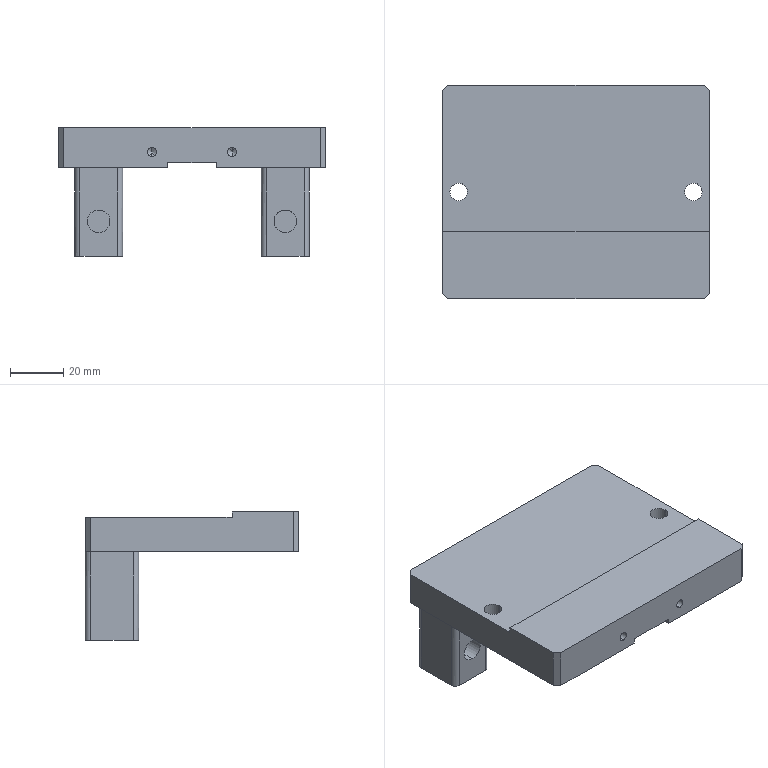NC program | NX | posted with a generic post | part box 100 x 80 x 48 mm
Whole program, first 1415 of 1793 lines:
N10 G17 G21 G94 G90
(FLOOR_WALL , TOOL : D80)
N12 T19 M6
N14 G54
N16 G17 G0 G90 X-95. Y41.997 S6500 M3
N18 G43 Z30. H19
N20 Z3.
N22 G94 G1 Z0. F1500.
N24 X-92.
N26 X92.
N28 Y15.999
N30 X-92.
N32 Y-10.
N34 X92.
N36 X95.
N38 Z3.
N40 G0 Z30.
N42 M5
(ZLEVEL_PROFILE , TOOL : D10)
N44 T15 M6
N46 G54
N48 G17 G0 G90 X47.703 Y-45.1 S9500 M3
N50 G43 Z30. H15
N52 Z1.5
N54 G94 G1 X0. Z-1. F1000.
N56 X-48. F3000.
N58 G2 X-51.606 Y-43.606 R5.1
N60 G1 X-53.606 Y-41.606
N62 G2 X-55.1 Y-38. R5.1
N64 G1 Y38.
N66 G2 X-53.606 Y41.606 R5.1
N68 G1 X-51.606 Y43.606
N70 G2 X-48. Y45.1 R5.1
N72 G1 X48.
N74 G2 X51.606 Y43.606 R5.1
N76 G1 X53.606 Y41.606
N78 G2 X55.1 Y38. R5.1
N80 G1 Y-38.
N82 G2 X53.606 Y-41.606 R5.1
N84 G1 X51.606 Y-43.606
N86 G2 X48. Y-45.1 R5.1
N88 G1 X0.
N90 X-48. Z-1.124
N92 X-48.5 Y-45.075 Z-1.125
N94 X-48.995 Y-45.002 Z-1.127
N96 X-49.48 Y-44.88 Z-1.128
N98 X-49.952 Y-44.712 Z-1.129
N100 X-50.404 Y-44.498 Z-1.13
N102 X-50.833 Y-44.24 Z-1.132
N104 X-51.235 Y-43.942 Z-1.133
N106 X-51.606 Y-43.606 Z-1.134
N108 X-53.606 Y-41.606 Z-1.142
N110 X-53.942 Y-41.235 Z-1.143
N112 X-54.24 Y-40.833 Z-1.144
N114 X-54.498 Y-40.404 Z-1.145
N116 X-54.712 Y-39.952 Z-1.147
N118 X-54.88 Y-39.48 Z-1.148
N120 X-55.002 Y-38.995 Z-1.149
N122 X-55.075 Y-38.5 Z-1.151
N124 X-55.1 Y-38. Z-1.152
N126 Y38. Z-1.348
N128 X-55.075 Y38.5 Z-1.349
N130 X-55.002 Y38.995 Z-1.351
N132 X-54.88 Y39.48 Z-1.352
N134 X-54.712 Y39.952 Z-1.353
N136 X-54.498 Y40.404 Z-1.355
N138 X-54.24 Y40.833 Z-1.356
N140 X-53.942 Y41.235 Z-1.357
N142 X-53.606 Y41.606 Z-1.358
N144 X-51.606 Y43.606 Z-1.366
N146 X-51.235 Y43.942 Z-1.367
N148 X-50.833 Y44.24 Z-1.368
N150 X-50.404 Y44.498 Z-1.37
N152 X-49.952 Y44.712 Z-1.371
N154 X-49.48 Y44.88 Z-1.372
N156 X-48.995 Y45.002 Z-1.373
N158 X-48.5 Y45.075 Z-1.375
N160 X-48. Y45.1 Z-1.376
N162 X48. Z-1.624
N164 X48.5 Y45.075 Z-1.625
N166 X48.995 Y45.002 Z-1.627
N168 X49.48 Y44.88 Z-1.628
N170 X49.952 Y44.712 Z-1.629
N172 X50.404 Y44.498 Z-1.63
N174 X50.833 Y44.24 Z-1.632
N176 X51.235 Y43.942 Z-1.633
N178 X51.606 Y43.606 Z-1.634
N180 X53.606 Y41.606 Z-1.642
N182 X53.942 Y41.235 Z-1.643
N184 X54.24 Y40.833 Z-1.644
N186 X54.498 Y40.404 Z-1.645
N188 X54.712 Y39.952 Z-1.647
N190 X54.88 Y39.48 Z-1.648
N192 X55.002 Y38.995 Z-1.649
N194 X55.075 Y38.5 Z-1.651
N196 X55.1 Y38. Z-1.652
N198 Y-38. Z-1.848
N200 X55.075 Y-38.5 Z-1.849
N202 X55.002 Y-38.995 Z-1.851
N204 X54.88 Y-39.48 Z-1.852
N206 X54.712 Y-39.952 Z-1.853
N208 X54.498 Y-40.404 Z-1.855
N210 X54.24 Y-40.833 Z-1.856
N212 X53.942 Y-41.235 Z-1.857
N214 X53.606 Y-41.606 Z-1.858
N216 X51.606 Y-43.606 Z-1.866
N218 X51.235 Y-43.942 Z-1.867
N220 X50.833 Y-44.24 Z-1.868
N222 X50.404 Y-44.498 Z-1.87
N224 X49.952 Y-44.712 Z-1.871
N226 X49.48 Y-44.88 Z-1.872
N228 X48.995 Y-45.002 Z-1.873
N230 X48.5 Y-45.075 Z-1.875
N232 X48. Y-45.1 Z-1.876
N234 X0. Z-2.
N236 X-48. Z-2.124
N238 X-48.5 Y-45.075 Z-2.125
N240 X-48.995 Y-45.002 Z-2.127
N242 X-49.48 Y-44.88 Z-2.128
N244 X-49.952 Y-44.712 Z-2.129
N246 X-50.404 Y-44.498 Z-2.13
N248 X-50.833 Y-44.24 Z-2.132
N250 X-51.235 Y-43.942 Z-2.133
N252 X-51.606 Y-43.606 Z-2.134
N254 X-53.606 Y-41.606 Z-2.142
N256 X-53.942 Y-41.235 Z-2.143
N258 X-54.24 Y-40.833 Z-2.144
N260 X-54.498 Y-40.404 Z-2.145
N262 X-54.712 Y-39.952 Z-2.147
N264 X-54.88 Y-39.48 Z-2.148
N266 X-55.002 Y-38.995 Z-2.149
N268 X-55.075 Y-38.5 Z-2.151
N270 X-55.1 Y-38. Z-2.152
N272 Y38. Z-2.348
N274 X-55.075 Y38.5 Z-2.349
N276 X-55.002 Y38.995 Z-2.351
N278 X-54.88 Y39.48 Z-2.352
N280 X-54.712 Y39.952 Z-2.353
N282 X-54.498 Y40.404 Z-2.355
N284 X-54.24 Y40.833 Z-2.356
N286 X-53.942 Y41.235 Z-2.357
N288 X-53.606 Y41.606 Z-2.358
N290 X-51.606 Y43.606 Z-2.366
N292 X-51.235 Y43.942 Z-2.367
N294 X-50.833 Y44.24 Z-2.368
N296 X-50.404 Y44.498 Z-2.37
N298 X-49.952 Y44.712 Z-2.371
N300 X-49.48 Y44.88 Z-2.372
N302 X-48.995 Y45.002 Z-2.373
N304 X-48.5 Y45.075 Z-2.375
N306 X-48. Y45.1 Z-2.376
N308 X48. Z-2.624
N310 X48.5 Y45.075 Z-2.625
N312 X48.995 Y45.002 Z-2.627
N314 X49.48 Y44.88 Z-2.628
N316 X49.952 Y44.712 Z-2.629
N318 X50.404 Y44.498 Z-2.63
N320 X50.833 Y44.24 Z-2.632
N322 X51.235 Y43.942 Z-2.633
N324 X51.606 Y43.606 Z-2.634
N326 X53.606 Y41.606 Z-2.642
N328 X53.942 Y41.235 Z-2.643
N330 X54.24 Y40.833 Z-2.644
N332 X54.498 Y40.404 Z-2.645
N334 X54.712 Y39.952 Z-2.647
N336 X54.88 Y39.48 Z-2.648
N338 X55.002 Y38.995 Z-2.649
N340 X55.075 Y38.5 Z-2.651
N342 X55.1 Y38. Z-2.652
N344 Y-38. Z-2.848
N346 X55.075 Y-38.5 Z-2.849
N348 X55.002 Y-38.995 Z-2.851
N350 X54.88 Y-39.48 Z-2.852
N352 X54.712 Y-39.952 Z-2.853
N354 X54.498 Y-40.404 Z-2.855
N356 X54.24 Y-40.833 Z-2.856
N358 X53.942 Y-41.235 Z-2.857
N360 X53.606 Y-41.606 Z-2.858
N362 X51.606 Y-43.606 Z-2.866
N364 X51.235 Y-43.942 Z-2.867
N366 X50.833 Y-44.24 Z-2.868
N368 X50.404 Y-44.498 Z-2.87
N370 X49.952 Y-44.712 Z-2.871
N372 X49.48 Y-44.88 Z-2.872
N374 X48.995 Y-45.002 Z-2.873
N376 X48.5 Y-45.075 Z-2.875
N378 X48. Y-45.1 Z-2.876
N380 X0. Z-3.
N382 X-48. Z-3.124
N384 X-48.5 Y-45.075 Z-3.125
N386 X-48.995 Y-45.002 Z-3.127
N388 X-49.48 Y-44.88 Z-3.128
N390 X-49.952 Y-44.712 Z-3.129
N392 X-50.404 Y-44.498 Z-3.13
N394 X-50.833 Y-44.24 Z-3.132
N396 X-51.235 Y-43.942 Z-3.133
N398 X-51.606 Y-43.606 Z-3.134
N400 X-53.606 Y-41.606 Z-3.142
N402 X-53.942 Y-41.235 Z-3.143
N404 X-54.24 Y-40.833 Z-3.144
N406 X-54.498 Y-40.404 Z-3.145
N408 X-54.712 Y-39.952 Z-3.147
N410 X-54.88 Y-39.48 Z-3.148
N412 X-55.002 Y-38.995 Z-3.149
N414 X-55.075 Y-38.5 Z-3.151
N416 X-55.1 Y-38. Z-3.152
N418 Y38. Z-3.348
N420 X-55.075 Y38.5 Z-3.349
N422 X-55.002 Y38.995 Z-3.351
N424 X-54.88 Y39.48 Z-3.352
N426 X-54.712 Y39.952 Z-3.353
N428 X-54.498 Y40.404 Z-3.355
N430 X-54.24 Y40.833 Z-3.356
N432 X-53.942 Y41.235 Z-3.357
N434 X-53.606 Y41.606 Z-3.358
N436 X-51.606 Y43.606 Z-3.366
N438 X-51.235 Y43.942 Z-3.367
N440 X-50.833 Y44.24 Z-3.368
N442 X-50.404 Y44.498 Z-3.37
N444 X-49.952 Y44.712 Z-3.371
N446 X-49.48 Y44.88 Z-3.372
N448 X-48.995 Y45.002 Z-3.373
N450 X-48.5 Y45.075 Z-3.375
N452 X-48. Y45.1 Z-3.376
N454 X48. Z-3.624
N456 X48.5 Y45.075 Z-3.625
N458 X48.995 Y45.002 Z-3.627
N460 X49.48 Y44.88 Z-3.628
N462 X49.952 Y44.712 Z-3.629
N464 X50.404 Y44.498 Z-3.63
N466 X50.833 Y44.24 Z-3.632
N468 X51.235 Y43.942 Z-3.633
N470 X51.606 Y43.606 Z-3.634
N472 X53.606 Y41.606 Z-3.642
N474 X53.942 Y41.235 Z-3.643
N476 X54.24 Y40.833 Z-3.644
N478 X54.498 Y40.404 Z-3.645
N480 X54.712 Y39.952 Z-3.647
N482 X54.88 Y39.48 Z-3.648
N484 X55.002 Y38.995 Z-3.649
N486 X55.075 Y38.5 Z-3.651
N488 X55.1 Y38. Z-3.652
N490 Y-38. Z-3.848
N492 X55.075 Y-38.5 Z-3.849
N494 X55.002 Y-38.995 Z-3.851
N496 X54.88 Y-39.48 Z-3.852
N498 X54.712 Y-39.952 Z-3.853
N500 X54.498 Y-40.404 Z-3.855
N502 X54.24 Y-40.833 Z-3.856
N504 X53.942 Y-41.235 Z-3.857
N506 X53.606 Y-41.606 Z-3.858
N508 X51.606 Y-43.606 Z-3.866
N510 X51.235 Y-43.942 Z-3.867
N512 X50.833 Y-44.24 Z-3.868
N514 X50.404 Y-44.498 Z-3.87
N516 X49.952 Y-44.712 Z-3.871
N518 X49.48 Y-44.88 Z-3.872
N520 X48.995 Y-45.002 Z-3.873
N522 X48.5 Y-45.075 Z-3.875
N524 X48. Y-45.1 Z-3.876
N526 X0. Z-4.
N528 X-48. Z-4.124
N530 X-48.5 Y-45.075 Z-4.125
N532 X-48.995 Y-45.002 Z-4.127
N534 X-49.48 Y-44.88 Z-4.128
N536 X-49.952 Y-44.712 Z-4.129
N538 X-50.404 Y-44.498 Z-4.13
N540 X-50.833 Y-44.24 Z-4.132
N542 X-51.235 Y-43.942 Z-4.133
N544 X-51.606 Y-43.606 Z-4.134
N546 X-53.606 Y-41.606 Z-4.142
N548 X-53.942 Y-41.235 Z-4.143
N550 X-54.24 Y-40.833 Z-4.144
N552 X-54.498 Y-40.404 Z-4.145
N554 X-54.712 Y-39.952 Z-4.147
N556 X-54.88 Y-39.48 Z-4.148
N558 X-55.002 Y-38.995 Z-4.149
N560 X-55.075 Y-38.5 Z-4.151
N562 X-55.1 Y-38. Z-4.152
N564 Y38. Z-4.348
N566 X-55.075 Y38.5 Z-4.349
N568 X-55.002 Y38.995 Z-4.351
N570 X-54.88 Y39.48 Z-4.352
N572 X-54.712 Y39.952 Z-4.353
N574 X-54.498 Y40.404 Z-4.355
N576 X-54.24 Y40.833 Z-4.356
N578 X-53.942 Y41.235 Z-4.357
N580 X-53.606 Y41.606 Z-4.358
N582 X-51.606 Y43.606 Z-4.366
N584 X-51.235 Y43.942 Z-4.367
N586 X-50.833 Y44.24 Z-4.368
N588 X-50.404 Y44.498 Z-4.37
N590 X-49.952 Y44.712 Z-4.371
N592 X-49.48 Y44.88 Z-4.372
N594 X-48.995 Y45.002 Z-4.373
N596 X-48.5 Y45.075 Z-4.375
N598 X-48. Y45.1 Z-4.376
N600 X48. Z-4.624
N602 X48.5 Y45.075 Z-4.625
N604 X48.995 Y45.002 Z-4.627
N606 X49.48 Y44.88 Z-4.628
N608 X49.952 Y44.712 Z-4.629
N610 X50.404 Y44.498 Z-4.63
N612 X50.833 Y44.24 Z-4.632
N614 X51.235 Y43.942 Z-4.633
N616 X51.606 Y43.606 Z-4.634
N618 X53.606 Y41.606 Z-4.642
N620 X53.942 Y41.235 Z-4.643
N622 X54.24 Y40.833 Z-4.644
N624 X54.498 Y40.404 Z-4.645
N626 X54.712 Y39.952 Z-4.647
N628 X54.88 Y39.48 Z-4.648
N630 X55.002 Y38.995 Z-4.649
N632 X55.075 Y38.5 Z-4.651
N634 X55.1 Y38. Z-4.652
N636 Y-38. Z-4.848
N638 X55.075 Y-38.5 Z-4.849
N640 X55.002 Y-38.995 Z-4.851
N642 X54.88 Y-39.48 Z-4.852
N644 X54.712 Y-39.952 Z-4.853
N646 X54.498 Y-40.404 Z-4.855
N648 X54.24 Y-40.833 Z-4.856
N650 X53.942 Y-41.235 Z-4.857
N652 X53.606 Y-41.606 Z-4.858
N654 X51.606 Y-43.606 Z-4.866
N656 X51.235 Y-43.942 Z-4.867
N658 X50.833 Y-44.24 Z-4.868
N660 X50.404 Y-44.498 Z-4.87
N662 X49.952 Y-44.712 Z-4.871
N664 X49.48 Y-44.88 Z-4.872
N666 X48.995 Y-45.002 Z-4.873
N668 X48.5 Y-45.075 Z-4.875
N670 X48. Y-45.1 Z-4.876
N672 X0. Z-5.
N674 X-48. Z-5.124
N676 X-48.5 Y-45.075 Z-5.125
N678 X-48.995 Y-45.002 Z-5.127
N680 X-49.48 Y-44.88 Z-5.128
N682 X-49.952 Y-44.712 Z-5.129
N684 X-50.404 Y-44.498 Z-5.13
N686 X-50.833 Y-44.24 Z-5.132
N688 X-51.235 Y-43.942 Z-5.133
N690 X-51.606 Y-43.606 Z-5.134
N692 X-53.606 Y-41.606 Z-5.142
N694 X-53.942 Y-41.235 Z-5.143
N696 X-54.24 Y-40.833 Z-5.144
N698 X-54.498 Y-40.404 Z-5.145
N700 X-54.712 Y-39.952 Z-5.147
N702 X-54.88 Y-39.48 Z-5.148
N704 X-55.002 Y-38.995 Z-5.149
N706 X-55.075 Y-38.5 Z-5.151
N708 X-55.1 Y-38. Z-5.152
N710 Y38. Z-5.348
N712 X-55.075 Y38.5 Z-5.349
N714 X-55.002 Y38.995 Z-5.351
N716 X-54.88 Y39.48 Z-5.352
N718 X-54.712 Y39.952 Z-5.353
N720 X-54.498 Y40.404 Z-5.355
N722 X-54.24 Y40.833 Z-5.356
N724 X-53.942 Y41.235 Z-5.357
N726 X-53.606 Y41.606 Z-5.358
N728 X-51.606 Y43.606 Z-5.366
N730 X-51.235 Y43.942 Z-5.367
N732 X-50.833 Y44.24 Z-5.368
N734 X-50.404 Y44.498 Z-5.37
N736 X-49.952 Y44.712 Z-5.371
N738 X-49.48 Y44.88 Z-5.372
N740 X-48.995 Y45.002 Z-5.373
N742 X-48.5 Y45.075 Z-5.375
N744 X-48. Y45.1 Z-5.376
N746 X48. Z-5.624
N748 X48.5 Y45.075 Z-5.625
N750 X48.995 Y45.002 Z-5.627
N752 X49.48 Y44.88 Z-5.628
N754 X49.952 Y44.712 Z-5.629
N756 X50.404 Y44.498 Z-5.63
N758 X50.833 Y44.24 Z-5.632
N760 X51.235 Y43.942 Z-5.633
N762 X51.606 Y43.606 Z-5.634
N764 X53.606 Y41.606 Z-5.642
N766 X53.942 Y41.235 Z-5.643
N768 X54.24 Y40.833 Z-5.644
N770 X54.498 Y40.404 Z-5.645
N772 X54.712 Y39.952 Z-5.647
N774 X54.88 Y39.48 Z-5.648
N776 X55.002 Y38.995 Z-5.649
N778 X55.075 Y38.5 Z-5.651
N780 X55.1 Y38. Z-5.652
N782 Y-38. Z-5.848
N784 X55.075 Y-38.5 Z-5.849
N786 X55.002 Y-38.995 Z-5.851
N788 X54.88 Y-39.48 Z-5.852
N790 X54.712 Y-39.952 Z-5.853
N792 X54.498 Y-40.404 Z-5.855
N794 X54.24 Y-40.833 Z-5.856
N796 X53.942 Y-41.235 Z-5.857
N798 X53.606 Y-41.606 Z-5.858
N800 X51.606 Y-43.606 Z-5.866
N802 X51.235 Y-43.942 Z-5.867
N804 X50.833 Y-44.24 Z-5.868
N806 X50.404 Y-44.498 Z-5.87
N808 X49.952 Y-44.712 Z-5.871
N810 X49.48 Y-44.88 Z-5.872
N812 X48.995 Y-45.002 Z-5.873
N814 X48.5 Y-45.075 Z-5.875
N816 X48. Y-45.1 Z-5.876
N818 X0. Z-6.
N820 X-48. Z-6.124
N822 X-48.5 Y-45.075 Z-6.125
N824 X-48.995 Y-45.002 Z-6.127
N826 X-49.48 Y-44.88 Z-6.128
N828 X-49.952 Y-44.712 Z-6.129
N830 X-50.404 Y-44.498 Z-6.13
N832 X-50.833 Y-44.24 Z-6.132
N834 X-51.235 Y-43.942 Z-6.133
N836 X-51.606 Y-43.606 Z-6.134
N838 X-53.606 Y-41.606 Z-6.142
N840 X-53.942 Y-41.235 Z-6.143
N842 X-54.24 Y-40.833 Z-6.144
N844 X-54.498 Y-40.404 Z-6.145
N846 X-54.712 Y-39.952 Z-6.147
N848 X-54.88 Y-39.48 Z-6.148
N850 X-55.002 Y-38.995 Z-6.149
N852 X-55.075 Y-38.5 Z-6.151
N854 X-55.1 Y-38. Z-6.152
N856 Y38. Z-6.348
N858 X-55.075 Y38.5 Z-6.349
N860 X-55.002 Y38.995 Z-6.351
N862 X-54.88 Y39.48 Z-6.352
N864 X-54.712 Y39.952 Z-6.353
N866 X-54.498 Y40.404 Z-6.355
N868 X-54.24 Y40.833 Z-6.356
N870 X-53.942 Y41.235 Z-6.357
N872 X-53.606 Y41.606 Z-6.358
N874 X-51.606 Y43.606 Z-6.366
N876 X-51.235 Y43.942 Z-6.367
N878 X-50.833 Y44.24 Z-6.368
N880 X-50.404 Y44.498 Z-6.37
N882 X-49.952 Y44.712 Z-6.371
N884 X-49.48 Y44.88 Z-6.372
N886 X-48.995 Y45.002 Z-6.373
N888 X-48.5 Y45.075 Z-6.375
N890 X-48. Y45.1 Z-6.376
N892 X48. Z-6.624
N894 X48.5 Y45.075 Z-6.625
N896 X48.995 Y45.002 Z-6.627
N898 X49.48 Y44.88 Z-6.628
N900 X49.952 Y44.712 Z-6.629
N902 X50.404 Y44.498 Z-6.63
N904 X50.833 Y44.24 Z-6.632
N906 X51.235 Y43.942 Z-6.633
N908 X51.606 Y43.606 Z-6.634
N910 X53.606 Y41.606 Z-6.642
N912 X53.942 Y41.235 Z-6.643
N914 X54.24 Y40.833 Z-6.644
N916 X54.498 Y40.404 Z-6.645
N918 X54.712 Y39.952 Z-6.647
N920 X54.88 Y39.48 Z-6.648
N922 X55.002 Y38.995 Z-6.649
N924 X55.075 Y38.5 Z-6.651
N926 X55.1 Y38. Z-6.652
N928 Y-38. Z-6.848
N930 X55.075 Y-38.5 Z-6.849
N932 X55.002 Y-38.995 Z-6.851
N934 X54.88 Y-39.48 Z-6.852
N936 X54.712 Y-39.952 Z-6.853
N938 X54.498 Y-40.404 Z-6.855
N940 X54.24 Y-40.833 Z-6.856
N942 X53.942 Y-41.235 Z-6.857
N944 X53.606 Y-41.606 Z-6.858
N946 X51.606 Y-43.606 Z-6.866
N948 X51.235 Y-43.942 Z-6.867
N950 X50.833 Y-44.24 Z-6.868
N952 X50.404 Y-44.498 Z-6.87
N954 X49.952 Y-44.712 Z-6.871
N956 X49.48 Y-44.88 Z-6.872
N958 X48.995 Y-45.002 Z-6.873
N960 X48.5 Y-45.075 Z-6.875
N962 X48. Y-45.1 Z-6.876
N964 X0. Z-7.
N966 X-48. Z-7.124
N968 X-48.5 Y-45.075 Z-7.125
N970 X-48.995 Y-45.002 Z-7.127
N972 X-49.48 Y-44.88 Z-7.128
N974 X-49.952 Y-44.712 Z-7.129
N976 X-50.404 Y-44.498 Z-7.13
N978 X-50.833 Y-44.24 Z-7.132
N980 X-51.235 Y-43.942 Z-7.133
N982 X-51.606 Y-43.606 Z-7.134
N984 X-53.606 Y-41.606 Z-7.142
N986 X-53.942 Y-41.235 Z-7.143
N988 X-54.24 Y-40.833 Z-7.144
N990 X-54.498 Y-40.404 Z-7.145
N992 X-54.712 Y-39.952 Z-7.147
N994 X-54.88 Y-39.48 Z-7.148
N996 X-55.002 Y-38.995 Z-7.149
N998 X-55.075 Y-38.5 Z-7.151
N1000 X-55.1 Y-38. Z-7.152
N1002 Y38. Z-7.348
N1004 X-55.075 Y38.5 Z-7.349
N1006 X-55.002 Y38.995 Z-7.351
N1008 X-54.88 Y39.48 Z-7.352
N1010 X-54.712 Y39.952 Z-7.353
N1012 X-54.498 Y40.404 Z-7.355
N1014 X-54.24 Y40.833 Z-7.356
N1016 X-53.942 Y41.235 Z-7.357
N1018 X-53.606 Y41.606 Z-7.358
N1020 X-51.606 Y43.606 Z-7.366
N1022 X-51.235 Y43.942 Z-7.367
N1024 X-50.833 Y44.24 Z-7.368
N1026 X-50.404 Y44.498 Z-7.37
N1028 X-49.952 Y44.712 Z-7.371
N1030 X-49.48 Y44.88 Z-7.372
N1032 X-48.995 Y45.002 Z-7.373
N1034 X-48.5 Y45.075 Z-7.375
N1036 X-48. Y45.1 Z-7.376
N1038 X48. Z-7.624
N1040 X48.5 Y45.075 Z-7.625
N1042 X48.995 Y45.002 Z-7.627
N1044 X49.48 Y44.88 Z-7.628
N1046 X49.952 Y44.712 Z-7.629
N1048 X50.404 Y44.498 Z-7.63
N1050 X50.833 Y44.24 Z-7.632
N1052 X51.235 Y43.942 Z-7.633
N1054 X51.606 Y43.606 Z-7.634
N1056 X53.606 Y41.606 Z-7.642
N1058 X53.942 Y41.235 Z-7.643
N1060 X54.24 Y40.833 Z-7.644
N1062 X54.498 Y40.404 Z-7.645
N1064 X54.712 Y39.952 Z-7.647
N1066 X54.88 Y39.48 Z-7.648
N1068 X55.002 Y38.995 Z-7.649
N1070 X55.075 Y38.5 Z-7.651
N1072 X55.1 Y38. Z-7.652
N1074 Y-38. Z-7.848
N1076 X55.075 Y-38.5 Z-7.849
N1078 X55.002 Y-38.995 Z-7.851
N1080 X54.88 Y-39.48 Z-7.852
N1082 X54.712 Y-39.952 Z-7.853
N1084 X54.498 Y-40.404 Z-7.855
N1086 X54.24 Y-40.833 Z-7.856
N1088 X53.942 Y-41.235 Z-7.857
N1090 X53.606 Y-41.606 Z-7.858
N1092 X51.606 Y-43.606 Z-7.866
N1094 X51.235 Y-43.942 Z-7.867
N1096 X50.833 Y-44.24 Z-7.868
N1098 X50.404 Y-44.498 Z-7.87
N1100 X49.952 Y-44.712 Z-7.871
N1102 X49.48 Y-44.88 Z-7.872
N1104 X48.995 Y-45.002 Z-7.873
N1106 X48.5 Y-45.075 Z-7.875
N1108 X48. Y-45.1 Z-7.876
N1110 X0. Z-8.
N1112 X-48. Z-8.124
N1114 X-48.5 Y-45.075 Z-8.125
N1116 X-48.995 Y-45.002 Z-8.127
N1118 X-49.48 Y-44.88 Z-8.128
N1120 X-49.952 Y-44.712 Z-8.129
N1122 X-50.404 Y-44.498 Z-8.13
N1124 X-50.833 Y-44.24 Z-8.132
N1126 X-51.235 Y-43.942 Z-8.133
N1128 X-51.606 Y-43.606 Z-8.134
N1130 X-53.606 Y-41.606 Z-8.142
N1132 X-53.942 Y-41.235 Z-8.143
N1134 X-54.24 Y-40.833 Z-8.144
N1136 X-54.498 Y-40.404 Z-8.145
N1138 X-54.712 Y-39.952 Z-8.147
N1140 X-54.88 Y-39.48 Z-8.148
N1142 X-55.002 Y-38.995 Z-8.149
N1144 X-55.075 Y-38.5 Z-8.151
N1146 X-55.1 Y-38. Z-8.152
N1148 Y38. Z-8.348
N1150 X-55.075 Y38.5 Z-8.349
N1152 X-55.002 Y38.995 Z-8.351
N1154 X-54.88 Y39.48 Z-8.352
N1156 X-54.712 Y39.952 Z-8.353
N1158 X-54.498 Y40.404 Z-8.355
N1160 X-54.24 Y40.833 Z-8.356
N1162 X-53.942 Y41.235 Z-8.357
N1164 X-53.606 Y41.606 Z-8.358
N1166 X-51.606 Y43.606 Z-8.366
N1168 X-51.235 Y43.942 Z-8.367
N1170 X-50.833 Y44.24 Z-8.368
N1172 X-50.404 Y44.498 Z-8.37
N1174 X-49.952 Y44.712 Z-8.371
N1176 X-49.48 Y44.88 Z-8.372
N1178 X-48.995 Y45.002 Z-8.373
N1180 X-48.5 Y45.075 Z-8.375
N1182 X-48. Y45.1 Z-8.376
N1184 X48. Z-8.624
N1186 X48.5 Y45.075 Z-8.625
N1188 X48.995 Y45.002 Z-8.627
N1190 X49.48 Y44.88 Z-8.628
N1192 X49.952 Y44.712 Z-8.629
N1194 X50.404 Y44.498 Z-8.63
N1196 X50.833 Y44.24 Z-8.632
N1198 X51.235 Y43.942 Z-8.633
N1200 X51.606 Y43.606 Z-8.634
N1202 X53.606 Y41.606 Z-8.642
N1204 X53.942 Y41.235 Z-8.643
N1206 X54.24 Y40.833 Z-8.644
N1208 X54.498 Y40.404 Z-8.645
N1210 X54.712 Y39.952 Z-8.647
N1212 X54.88 Y39.48 Z-8.648
N1214 X55.002 Y38.995 Z-8.649
N1216 X55.075 Y38.5 Z-8.651
N1218 X55.1 Y38. Z-8.652
N1220 Y-38. Z-8.848
N1222 X55.075 Y-38.5 Z-8.849
N1224 X55.002 Y-38.995 Z-8.851
N1226 X54.88 Y-39.48 Z-8.852
N1228 X54.712 Y-39.952 Z-8.853
N1230 X54.498 Y-40.404 Z-8.855
N1232 X54.24 Y-40.833 Z-8.856
N1234 X53.942 Y-41.235 Z-8.857
N1236 X53.606 Y-41.606 Z-8.858
N1238 X51.606 Y-43.606 Z-8.866
N1240 X51.235 Y-43.942 Z-8.867
N1242 X50.833 Y-44.24 Z-8.868
N1244 X50.404 Y-44.498 Z-8.87
N1246 X49.952 Y-44.712 Z-8.871
N1248 X49.48 Y-44.88 Z-8.872
N1250 X48.995 Y-45.002 Z-8.873
N1252 X48.5 Y-45.075 Z-8.875
N1254 X48. Y-45.1 Z-8.876
N1256 X0. Z-9.
N1258 X-48. Z-9.124
N1260 X-48.5 Y-45.075 Z-9.125
N1262 X-48.995 Y-45.002 Z-9.127
N1264 X-49.48 Y-44.88 Z-9.128
N1266 X-49.952 Y-44.712 Z-9.129
N1268 X-50.404 Y-44.498 Z-9.13
N1270 X-50.833 Y-44.24 Z-9.132
N1272 X-51.235 Y-43.942 Z-9.133
N1274 X-51.606 Y-43.606 Z-9.134
N1276 X-53.606 Y-41.606 Z-9.142
N1278 X-53.942 Y-41.235 Z-9.143
N1280 X-54.24 Y-40.833 Z-9.144
N1282 X-54.498 Y-40.404 Z-9.145
N1284 X-54.712 Y-39.952 Z-9.147
N1286 X-54.88 Y-39.48 Z-9.148
N1288 X-55.002 Y-38.995 Z-9.149
N1290 X-55.075 Y-38.5 Z-9.151
N1292 X-55.1 Y-38. Z-9.152
N1294 Y38. Z-9.348
N1296 X-55.075 Y38.5 Z-9.349
N1298 X-55.002 Y38.995 Z-9.351
N1300 X-54.88 Y39.48 Z-9.352
N1302 X-54.712 Y39.952 Z-9.353
N1304 X-54.498 Y40.404 Z-9.355
N1306 X-54.24 Y40.833 Z-9.356
N1308 X-53.942 Y41.235 Z-9.357
N1310 X-53.606 Y41.606 Z-9.358
N1312 X-51.606 Y43.606 Z-9.366
N1314 X-51.235 Y43.942 Z-9.367
N1316 X-50.833 Y44.24 Z-9.368
N1318 X-50.404 Y44.498 Z-9.37
N1320 X-49.952 Y44.712 Z-9.371
N1322 X-49.48 Y44.88 Z-9.372
N1324 X-48.995 Y45.002 Z-9.373
N1326 X-48.5 Y45.075 Z-9.375
N1328 X-48. Y45.1 Z-9.376
N1330 X48. Z-9.624
N1332 X48.5 Y45.075 Z-9.625
N1334 X48.995 Y45.002 Z-9.627
N1336 X49.48 Y44.88 Z-9.628
N1338 X49.952 Y44.712 Z-9.629
N1340 X50.404 Y44.498 Z-9.63
N1342 X50.833 Y44.24 Z-9.632
N1344 X51.235 Y43.942 Z-9.633
N1346 X51.606 Y43.606 Z-9.634
N1348 X53.606 Y41.606 Z-9.642
N1350 X53.942 Y41.235 Z-9.643
N1352 X54.24 Y40.833 Z-9.644
N1354 X54.498 Y40.404 Z-9.645
N1356 X54.712 Y39.952 Z-9.647
N1358 X54.88 Y39.48 Z-9.648
N1360 X55.002 Y38.995 Z-9.649
N1362 X55.075 Y38.5 Z-9.651
N1364 X55.1 Y38. Z-9.652
N1366 Y-38. Z-9.848
N1368 X55.075 Y-38.5 Z-9.849
N1370 X55.002 Y-38.995 Z-9.851
N1372 X54.88 Y-39.48 Z-9.852
N1374 X54.712 Y-39.952 Z-9.853
N1376 X54.498 Y-40.404 Z-9.855
N1378 X54.24 Y-40.833 Z-9.856
N1380 X53.942 Y-41.235 Z-9.857
N1382 X53.606 Y-41.606 Z-9.858
N1384 X51.606 Y-43.606 Z-9.866
N1386 X51.235 Y-43.942 Z-9.867
N1388 X50.833 Y-44.24 Z-9.868
N1390 X50.404 Y-44.498 Z-9.87
N1392 X49.952 Y-44.712 Z-9.871
N1394 X49.48 Y-44.88 Z-9.872
N1396 X48.995 Y-45.002 Z-9.873
N1398 X48.5 Y-45.075 Z-9.875
N1400 X48. Y-45.1 Z-9.876
N1402 X0. Z-10.
N1404 X-48. Z-10.124
N1406 X-48.5 Y-45.075 Z-10.125
N1408 X-48.995 Y-45.002 Z-10.127
N1410 X-49.48 Y-44.88 Z-10.128
N1412 X-49.952 Y-44.712 Z-10.129
N1414 X-50.404 Y-44.498 Z-10.13
N1416 X-50.833 Y-44.24 Z-10.132
N1418 X-51.235 Y-43.942 Z-10.133
N1420 X-51.606 Y-43.606 Z-10.134
N1422 X-53.606 Y-41.606 Z-10.142
N1424 X-53.942 Y-41.235 Z-10.143
N1426 X-54.24 Y-40.833 Z-10.144
N1428 X-54.498 Y-40.404 Z-10.145
N1430 X-54.712 Y-39.952 Z-10.147
N1432 X-54.88 Y-39.48 Z-10.148
N1434 X-55.002 Y-38.995 Z-10.149
N1436 X-55.075 Y-38.5 Z-10.151
N1438 X-55.1 Y-38. Z-10.152
N1440 Y38. Z-10.348
N1442 X-55.075 Y38.5 Z-10.349
N1444 X-55.002 Y38.995 Z-10.351
N1446 X-54.88 Y39.48 Z-10.352
N1448 X-54.712 Y39.952 Z-10.353
N1450 X-54.498 Y40.404 Z-10.355
N1452 X-54.24 Y40.833 Z-10.356
N1454 X-53.942 Y41.235 Z-10.357
N1456 X-53.606 Y41.606 Z-10.358
N1458 X-51.606 Y43.606 Z-10.366
N1460 X-51.235 Y43.942 Z-10.367
N1462 X-50.833 Y44.24 Z-10.368
N1464 X-50.404 Y44.498 Z-10.37
N1466 X-49.952 Y44.712 Z-10.371
N1468 X-49.48 Y44.88 Z-10.372
N1470 X-48.995 Y45.002 Z-10.373
N1472 X-48.5 Y45.075 Z-10.375
N1474 X-48. Y45.1 Z-10.376
N1476 X48. Z-10.624
N1478 X48.5 Y45.075 Z-10.625
N1480 X48.995 Y45.002 Z-10.627
N1482 X49.48 Y44.88 Z-10.628
N1484 X49.952 Y44.712 Z-10.629
N1486 X50.404 Y44.498 Z-10.63
N1488 X50.833 Y44.24 Z-10.632
N1490 X51.235 Y43.942 Z-10.633
N1492 X51.606 Y43.606 Z-10.634
N1494 X53.606 Y41.606 Z-10.642
N1496 X53.942 Y41.235 Z-10.643
N1498 X54.24 Y40.833 Z-10.644
N1500 X54.498 Y40.404 Z-10.645
N1502 X54.712 Y39.952 Z-10.647
N1504 X54.88 Y39.48 Z-10.648
N1506 X55.002 Y38.995 Z-10.649
N1508 X55.075 Y38.5 Z-10.651
N1510 X55.1 Y38. Z-10.652
N1512 Y-38. Z-10.848
N1514 X55.075 Y-38.5 Z-10.849
N1516 X55.002 Y-38.995 Z-10.851
N1518 X54.88 Y-39.48 Z-10.852
N1520 X54.712 Y-39.952 Z-10.853
N1522 X54.498 Y-40.404 Z-10.855
N1524 X54.24 Y-40.833 Z-10.856
N1526 X53.942 Y-41.235 Z-10.857
N1528 X53.606 Y-41.606 Z-10.858
N1530 X51.606 Y-43.606 Z-10.866
N1532 X51.235 Y-43.942 Z-10.867
N1534 X50.833 Y-44.24 Z-10.868
N1536 X50.404 Y-44.498 Z-10.87
N1538 X49.952 Y-44.712 Z-10.871
N1540 X49.48 Y-44.88 Z-10.872
N1542 X48.995 Y-45.002 Z-10.873
N1544 X48.5 Y-45.075 Z-10.875
N1546 X48. Y-45.1 Z-10.876
N1548 X0. Z-11.
N1550 X-48. Z-11.124
N1552 X-48.5 Y-45.075 Z-11.125
N1554 X-48.995 Y-45.002 Z-11.127
N1556 X-49.48 Y-44.88 Z-11.128
N1558 X-49.952 Y-44.712 Z-11.129
N1560 X-50.404 Y-44.498 Z-11.13
N1562 X-50.833 Y-44.24 Z-11.132
N1564 X-51.235 Y-43.942 Z-11.133
N1566 X-51.606 Y-43.606 Z-11.134
N1568 X-53.606 Y-41.606 Z-11.142
N1570 X-53.942 Y-41.235 Z-11.143
N1572 X-54.24 Y-40.833 Z-11.144
N1574 X-54.498 Y-40.404 Z-11.145
N1576 X-54.712 Y-39.952 Z-11.147
N1578 X-54.88 Y-39.48 Z-11.148
N1580 X-55.002 Y-38.995 Z-11.149
N1582 X-55.075 Y-38.5 Z-11.151
N1584 X-55.1 Y-38. Z-11.152
N1586 Y38. Z-11.348
N1588 X-55.075 Y38.5 Z-11.349
N1590 X-55.002 Y38.995 Z-11.351
N1592 X-54.88 Y39.48 Z-11.352
N1594 X-54.712 Y39.952 Z-11.353
N1596 X-54.498 Y40.404 Z-11.355
N1598 X-54.24 Y40.833 Z-11.356
N1600 X-53.942 Y41.235 Z-11.357
N1602 X-53.606 Y41.606 Z-11.358
N1604 X-51.606 Y43.606 Z-11.366
N1606 X-51.235 Y43.942 Z-11.367
N1608 X-50.833 Y44.24 Z-11.368
N1610 X-50.404 Y44.498 Z-11.37
N1612 X-49.952 Y44.712 Z-11.371
N1614 X-49.48 Y44.88 Z-11.372
N1616 X-48.995 Y45.002 Z-11.373
N1618 X-48.5 Y45.075 Z-11.375
N1620 X-48. Y45.1 Z-11.376
N1622 X48. Z-11.624
N1624 X48.5 Y45.075 Z-11.625
N1626 X48.995 Y45.002 Z-11.627
N1628 X49.48 Y44.88 Z-11.628
N1630 X49.952 Y44.712 Z-11.629
N1632 X50.404 Y44.498 Z-11.63
N1634 X50.833 Y44.24 Z-11.632
N1636 X51.235 Y43.942 Z-11.633
N1638 X51.606 Y43.606 Z-11.634
N1640 X53.606 Y41.606 Z-11.642
N1642 X53.942 Y41.235 Z-11.643
N1644 X54.24 Y40.833 Z-11.644
N1646 X54.498 Y40.404 Z-11.645
N1648 X54.712 Y39.952 Z-11.647
N1650 X54.88 Y39.48 Z-11.648
N1652 X55.002 Y38.995 Z-11.649
N1654 X55.075 Y38.5 Z-11.651
N1656 X55.1 Y38. Z-11.652
N1658 Y-38. Z-11.848
N1660 X55.075 Y-38.5 Z-11.849
N1662 X55.002 Y-38.995 Z-11.851
N1664 X54.88 Y-39.48 Z-11.852
N1666 X54.712 Y-39.952 Z-11.853
N1668 X54.498 Y-40.404 Z-11.855
N1670 X54.24 Y-40.833 Z-11.856
N1672 X53.942 Y-41.235 Z-11.857
N1674 X53.606 Y-41.606 Z-11.858
N1676 X51.606 Y-43.606 Z-11.866
N1678 X51.235 Y-43.942 Z-11.867
N1680 X50.833 Y-44.24 Z-11.868
N1682 X50.404 Y-44.498 Z-11.87
N1684 X49.952 Y-44.712 Z-11.871
N1686 X49.48 Y-44.88 Z-11.872
N1688 X48.995 Y-45.002 Z-11.873
N1690 X48.5 Y-45.075 Z-11.875
N1692 X48. Y-45.1 Z-11.876
N1694 X0. Z-12.
N1696 X-48. Z-12.124
N1698 X-48.5 Y-45.075 Z-12.125
N1700 X-48.995 Y-45.002 Z-12.127
N1702 X-49.48 Y-44.88 Z-12.128
N1704 X-49.952 Y-44.712 Z-12.129
N1706 X-50.404 Y-44.498 Z-12.13
N1708 X-50.833 Y-44.24 Z-12.132
N1710 X-51.235 Y-43.942 Z-12.133
N1712 X-51.606 Y-43.606 Z-12.134
N1714 X-53.606 Y-41.606 Z-12.142
N1716 X-53.942 Y-41.235 Z-12.143
N1718 X-54.24 Y-40.833 Z-12.144
N1720 X-54.498 Y-40.404 Z-12.145
N1722 X-54.712 Y-39.952 Z-12.147
N1724 X-54.88 Y-39.48 Z-12.148
N1726 X-55.002 Y-38.995 Z-12.149
N1728 X-55.075 Y-38.5 Z-12.151
N1730 X-55.1 Y-38. Z-12.152
N1732 Y38. Z-12.348
N1734 X-55.075 Y38.5 Z-12.349
N1736 X-55.002 Y38.995 Z-12.351
N1738 X-54.88 Y39.48 Z-12.352
N1740 X-54.712 Y39.952 Z-12.353
N1742 X-54.498 Y40.404 Z-12.355
N1744 X-54.24 Y40.833 Z-12.356
N1746 X-53.942 Y41.235 Z-12.357
N1748 X-53.606 Y41.606 Z-12.358
N1750 X-51.606 Y43.606 Z-12.366
N1752 X-51.235 Y43.942 Z-12.367
N1754 X-50.833 Y44.24 Z-12.368
N1756 X-50.404 Y44.498 Z-12.37
N1758 X-49.952 Y44.712 Z-12.371
N1760 X-49.48 Y44.88 Z-12.372
N1762 X-48.995 Y45.002 Z-12.373
N1764 X-48.5 Y45.075 Z-12.375
N1766 X-48. Y45.1 Z-12.376
N1768 X48. Z-12.624
N1770 X48.5 Y45.075 Z-12.625
N1772 X48.995 Y45.002 Z-12.627
N1774 X49.48 Y44.88 Z-12.628
N1776 X49.952 Y44.712 Z-12.629
N1778 X50.404 Y44.498 Z-12.63
N1780 X50.833 Y44.24 Z-12.632
N1782 X51.235 Y43.942 Z-12.633
N1784 X51.606 Y43.606 Z-12.634
N1786 X53.606 Y41.606 Z-12.642
N1788 X53.942 Y41.235 Z-12.643
N1790 X54.24 Y40.833 Z-12.644
N1792 X54.498 Y40.404 Z-12.645
N1794 X54.712 Y39.952 Z-12.647
N1796 X54.88 Y39.48 Z-12.648
N1798 X55.002 Y38.995 Z-12.649
N1800 X55.075 Y38.5 Z-12.651
N1802 X55.1 Y38. Z-12.652
N1804 Y-38. Z-12.848
N1806 X55.075 Y-38.5 Z-12.849
N1808 X55.002 Y-38.995 Z-12.851
N1810 X54.88 Y-39.48 Z-12.852
N1812 X54.712 Y-39.952 Z-12.853
N1814 X54.498 Y-40.404 Z-12.855
N1816 X54.24 Y-40.833 Z-12.856
N1818 X53.942 Y-41.235 Z-12.857
N1820 X53.606 Y-41.606 Z-12.858
N1822 X51.606 Y-43.606 Z-12.866
N1824 X51.235 Y-43.942 Z-12.867
N1826 X50.833 Y-44.24 Z-12.868
N1828 X50.404 Y-44.498 Z-12.87
N1830 X49.952 Y-44.712 Z-12.871
N1832 X49.48 Y-44.88 Z-12.872
N1834 X48.995 Y-45.002 Z-12.873
N1836 X48.5 Y-45.075 Z-12.875
N1838 X48. Y-45.1 Z-12.876
N1840 X0. Z-13.
N1842 X-48. Z-13.124
N1844 X-48.5 Y-45.075 Z-13.125
N1846 X-48.995 Y-45.002 Z-13.127
N1848 X-49.48 Y-44.88 Z-13.128
N1850 X-49.952 Y-44.712 Z-13.129
N1852 X-50.404 Y-44.498 Z-13.13
N1854 X-50.833 Y-44.24 Z-13.132
N1856 X-51.235 Y-43.942 Z-13.133
N1858 X-51.606 Y-43.606 Z-13.134
N1860 X-53.606 Y-41.606 Z-13.142
N1862 X-53.942 Y-41.235 Z-13.143
N1864 X-54.24 Y-40.833 Z-13.144
N1866 X-54.498 Y-40.404 Z-13.145
N1868 X-54.712 Y-39.952 Z-13.147
N1870 X-54.88 Y-39.48 Z-13.148
N1872 X-55.002 Y-38.995 Z-13.149
N1874 X-55.075 Y-38.5 Z-13.151
N1876 X-55.1 Y-38. Z-13.152
N1878 Y38. Z-13.348
N1880 X-55.075 Y38.5 Z-13.349
N1882 X-55.002 Y38.995 Z-13.351
N1884 X-54.88 Y39.48 Z-13.352
N1886 X-54.712 Y39.952 Z-13.353
N1888 X-54.498 Y40.404 Z-13.355
N1890 X-54.24 Y40.833 Z-13.356
N1892 X-53.942 Y41.235 Z-13.357
N1894 X-53.606 Y41.606 Z-13.358
N1896 X-51.606 Y43.606 Z-13.366
N1898 X-51.235 Y43.942 Z-13.367
N1900 X-50.833 Y44.24 Z-13.368
N1902 X-50.404 Y44.498 Z-13.37
N1904 X-49.952 Y44.712 Z-13.371
N1906 X-49.48 Y44.88 Z-13.372
N1908 X-48.995 Y45.002 Z-13.373
N1910 X-48.5 Y45.075 Z-13.375
N1912 X-48. Y45.1 Z-13.376
N1914 X48. Z-13.624
N1916 X48.5 Y45.075 Z-13.625
N1918 X48.995 Y45.002 Z-13.627
N1920 X49.48 Y44.88 Z-13.628
N1922 X49.952 Y44.712 Z-13.629
N1924 X50.404 Y44.498 Z-13.63
N1926 X50.833 Y44.24 Z-13.632
N1928 X51.235 Y43.942 Z-13.633
N1930 X51.606 Y43.606 Z-13.634
N1932 X53.606 Y41.606 Z-13.642
N1934 X53.942 Y41.235 Z-13.643
N1936 X54.24 Y40.833 Z-13.644
N1938 X54.498 Y40.404 Z-13.645
N1940 X54.712 Y39.952 Z-13.647
N1942 X54.88 Y39.48 Z-13.648
N1944 X55.002 Y38.995 Z-13.649
N1946 X55.075 Y38.5 Z-13.651
N1948 X55.1 Y38. Z-13.652
N1950 Y-38. Z-13.848
N1952 X55.075 Y-38.5 Z-13.849
N1954 X55.002 Y-38.995 Z-13.851
N1956 X54.88 Y-39.48 Z-13.852
N1958 X54.712 Y-39.952 Z-13.853
N1960 X54.498 Y-40.404 Z-13.855
N1962 X54.24 Y-40.833 Z-13.856
N1964 X53.942 Y-41.235 Z-13.857
N1966 X53.606 Y-41.606 Z-13.858
N1968 X51.606 Y-43.606 Z-13.866
N1970 X51.235 Y-43.942 Z-13.867
N1972 X50.833 Y-44.24 Z-13.868
N1974 X50.404 Y-44.498 Z-13.87
N1976 X49.952 Y-44.712 Z-13.871
N1978 X49.48 Y-44.88 Z-13.872
N1980 X48.995 Y-45.002 Z-13.873
N1982 X48.5 Y-45.075 Z-13.875
N1984 X48. Y-45.1 Z-13.876
N1986 X0. Z-14.
N1988 X-48. Z-14.124
N1990 X-48.5 Y-45.075 Z-14.125
N1992 X-48.995 Y-45.002 Z-14.127
N1994 X-49.48 Y-44.88 Z-14.128
N1996 X-49.952 Y-44.712 Z-14.129
N1998 X-50.404 Y-44.498 Z-14.13
N2000 X-50.833 Y-44.24 Z-14.132
N2002 X-51.235 Y-43.942 Z-14.133
N2004 X-51.606 Y-43.606 Z-14.134
N2006 X-53.606 Y-41.606 Z-14.142
N2008 X-53.942 Y-41.235 Z-14.143
N2010 X-54.24 Y-40.833 Z-14.144
N2012 X-54.498 Y-40.404 Z-14.145
N2014 X-54.712 Y-39.952 Z-14.147
N2016 X-54.88 Y-39.48 Z-14.148
N2018 X-55.002 Y-38.995 Z-14.149
N2020 X-55.075 Y-38.5 Z-14.151
N2022 X-55.1 Y-38. Z-14.152
N2024 Y38. Z-14.348
N2026 X-55.075 Y38.5 Z-14.349
N2028 X-55.002 Y38.995 Z-14.351
N2030 X-54.88 Y39.48 Z-14.352
N2032 X-54.712 Y39.952 Z-14.353
N2034 X-54.498 Y40.404 Z-14.355
N2036 X-54.24 Y40.833 Z-14.356
N2038 X-53.942 Y41.235 Z-14.357
N2040 X-53.606 Y41.606 Z-14.358
N2042 X-51.606 Y43.606 Z-14.366
N2044 X-51.235 Y43.942 Z-14.367
N2046 X-50.833 Y44.24 Z-14.368
N2048 X-50.404 Y44.498 Z-14.37
N2050 X-49.952 Y44.712 Z-14.371
N2052 X-49.48 Y44.88 Z-14.372
N2054 X-48.995 Y45.002 Z-14.373
N2056 X-48.5 Y45.075 Z-14.375
N2058 X-48. Y45.1 Z-14.376
N2060 X48. Z-14.624
N2062 X48.5 Y45.075 Z-14.625
N2064 X48.995 Y45.002 Z-14.627
N2066 X49.48 Y44.88 Z-14.628
N2068 X49.952 Y44.712 Z-14.629
N2070 X50.404 Y44.498 Z-14.63
N2072 X50.833 Y44.24 Z-14.632
N2074 X51.235 Y43.942 Z-14.633
N2076 X51.606 Y43.606 Z-14.634
N2078 X53.606 Y41.606 Z-14.642
N2080 X53.942 Y41.235 Z-14.643
N2082 X54.24 Y40.833 Z-14.644
N2084 X54.498 Y40.404 Z-14.645
N2086 X54.712 Y39.952 Z-14.647
N2088 X54.88 Y39.48 Z-14.648
N2090 X55.002 Y38.995 Z-14.649
N2092 X55.075 Y38.5 Z-14.651
N2094 X55.1 Y38. Z-14.652
N2096 Y-38. Z-14.848
N2098 X55.075 Y-38.5 Z-14.849
N2100 X55.002 Y-38.995 Z-14.851
N2102 X54.88 Y-39.48 Z-14.852
N2104 X54.712 Y-39.952 Z-14.853
N2106 X54.498 Y-40.404 Z-14.855
N2108 X54.24 Y-40.833 Z-14.856
N2110 X53.942 Y-41.235 Z-14.857
N2112 X53.606 Y-41.606 Z-14.858
N2114 X51.606 Y-43.606 Z-14.866
N2116 X51.235 Y-43.942 Z-14.867
N2118 X50.833 Y-44.24 Z-14.868
N2120 X50.404 Y-44.498 Z-14.87
N2122 X49.952 Y-44.712 Z-14.871
N2124 X49.48 Y-44.88 Z-14.872
N2126 X48.995 Y-45.002 Z-14.873
N2128 X48.5 Y-45.075 Z-14.875
N2130 X48. Y-45.1 Z-14.876
N2132 X0. Z-15.
N2134 X-48. Z-15.124
N2136 X-48.5 Y-45.075 Z-15.125
N2138 X-48.995 Y-45.002 Z-15.127
N2140 X-49.48 Y-44.88 Z-15.128
N2142 X-49.952 Y-44.712 Z-15.129
N2144 X-50.404 Y-44.498 Z-15.13
N2146 X-50.833 Y-44.24 Z-15.132
N2148 X-51.235 Y-43.942 Z-15.133
N2150 X-51.606 Y-43.606 Z-15.134
N2152 X-53.606 Y-41.606 Z-15.142
N2154 X-53.942 Y-41.235 Z-15.143
N2156 X-54.24 Y-40.833 Z-15.144
N2158 X-54.498 Y-40.404 Z-15.145
N2160 X-54.712 Y-39.952 Z-15.147
N2162 X-54.88 Y-39.48 Z-15.148
N2164 X-55.002 Y-38.995 Z-15.149
N2166 X-55.075 Y-38.5 Z-15.151
N2168 X-55.1 Y-38. Z-15.152
N2170 Y38. Z-15.348
N2172 X-55.075 Y38.5 Z-15.349
N2174 X-55.002 Y38.995 Z-15.351
N2176 X-54.88 Y39.48 Z-15.352
N2178 X-54.712 Y39.952 Z-15.353
N2180 X-54.498 Y40.404 Z-15.355
N2182 X-54.24 Y40.833 Z-15.356
N2184 X-53.942 Y41.235 Z-15.357
N2186 X-53.606 Y41.606 Z-15.358
N2188 X-51.606 Y43.606 Z-15.366
N2190 X-51.235 Y43.942 Z-15.367
N2192 X-50.833 Y44.24 Z-15.368
N2194 X-50.404 Y44.498 Z-15.37
N2196 X-49.952 Y44.712 Z-15.371
N2198 X-49.48 Y44.88 Z-15.372
N2200 X-48.995 Y45.002 Z-15.373
N2202 X-48.5 Y45.075 Z-15.375
N2204 X-48. Y45.1 Z-15.376
N2206 X48. Z-15.624
N2208 X48.5 Y45.075 Z-15.625
N2210 X48.995 Y45.002 Z-15.627
N2212 X49.48 Y44.88 Z-15.628
N2214 X49.952 Y44.712 Z-15.629
N2216 X50.404 Y44.498 Z-15.63
N2218 X50.833 Y44.24 Z-15.632
N2220 X51.235 Y43.942 Z-15.633
N2222 X51.606 Y43.606 Z-15.634
N2224 X53.606 Y41.606 Z-15.642
N2226 X53.942 Y41.235 Z-15.643
N2228 X54.24 Y40.833 Z-15.644
N2230 X54.498 Y40.404 Z-15.645
N2232 X54.712 Y39.952 Z-15.647
N2234 X54.88 Y39.48 Z-15.648
N2236 X55.002 Y38.995 Z-15.649
N2238 X55.075 Y38.5 Z-15.651
N2240 X55.1 Y38. Z-15.652
N2242 Y-38. Z-15.848
N2244 X55.075 Y-38.5 Z-15.849
N2246 X55.002 Y-38.995 Z-15.851
N2248 X54.88 Y-39.48 Z-15.852
N2250 X54.712 Y-39.952 Z-15.853
N2252 X54.498 Y-40.404 Z-15.855
N2254 X54.24 Y-40.833 Z-15.856
N2256 X53.942 Y-41.235 Z-15.857
N2258 X53.606 Y-41.606 Z-15.858
N2260 X51.606 Y-43.606 Z-15.866
N2262 X51.235 Y-43.942 Z-15.867
N2264 X50.833 Y-44.24 Z-15.868
N2266 X50.404 Y-44.498 Z-15.87
N2268 X49.952 Y-44.712 Z-15.871
N2270 X49.48 Y-44.88 Z-15.872
N2272 X48.995 Y-45.002 Z-15.873
N2274 X48.5 Y-45.075 Z-15.875
N2276 X48. Y-45.1 Z-15.876
N2278 X0. Z-16.
N2280 X-48. Z-16.124
N2282 X-48.5 Y-45.075 Z-16.125
N2284 X-48.995 Y-45.002 Z-16.127
N2286 X-49.48 Y-44.88 Z-16.128
N2288 X-49.952 Y-44.712 Z-16.129
N2290 X-50.404 Y-44.498 Z-16.13
N2292 X-50.833 Y-44.24 Z-16.132
N2294 X-51.235 Y-43.942 Z-16.133
N2296 X-51.606 Y-43.606 Z-16.134
N2298 X-53.606 Y-41.606 Z-16.142
N2300 X-53.942 Y-41.235 Z-16.143
N2302 X-54.24 Y-40.833 Z-16.144
N2304 X-54.498 Y-40.404 Z-16.145
N2306 X-54.712 Y-39.952 Z-16.147
N2308 X-54.88 Y-39.48 Z-16.148
N2310 X-55.002 Y-38.995 Z-16.149
N2312 X-55.075 Y-38.5 Z-16.151
N2314 X-55.1 Y-38. Z-16.152
N2316 Y38. Z-16.348
N2318 X-55.075 Y38.5 Z-16.349
N2320 X-55.002 Y38.995 Z-16.351
N2322 X-54.88 Y39.48 Z-16.352
N2324 X-54.712 Y39.952 Z-16.353
N2326 X-54.498 Y40.404 Z-16.355
N2328 X-54.24 Y40.833 Z-16.356
N2330 X-53.942 Y41.235 Z-16.357
N2332 X-53.606 Y41.606 Z-16.358
N2334 X-51.606 Y43.606 Z-16.366
N2336 X-51.235 Y43.942 Z-16.367
N2338 X-50.833 Y44.24 Z-16.368
N2340 X-50.404 Y44.498 Z-16.37
N2342 X-49.952 Y44.712 Z-16.371
N2344 X-49.48 Y44.88 Z-16.372
N2346 X-48.995 Y45.002 Z-16.373
N2348 X-48.5 Y45.075 Z-16.375
N2350 X-48. Y45.1 Z-16.376
N2352 X48. Z-16.624
N2354 X48.5 Y45.075 Z-16.625
N2356 X48.995 Y45.002 Z-16.627
N2358 X49.48 Y44.88 Z-16.628
N2360 X49.952 Y44.712 Z-16.629
N2362 X50.404 Y44.498 Z-16.63
N2364 X50.833 Y44.24 Z-16.632
N2366 X51.235 Y43.942 Z-16.633
N2368 X51.606 Y43.606 Z-16.634
N2370 X53.606 Y41.606 Z-16.642
N2372 X53.942 Y41.235 Z-16.643
N2374 X54.24 Y40.833 Z-16.644
N2376 X54.498 Y40.404 Z-16.645
N2378 X54.712 Y39.952 Z-16.647
N2380 X54.88 Y39.48 Z-16.648
N2382 X55.002 Y38.995 Z-16.649
N2384 X55.075 Y38.5 Z-16.651
N2386 X55.1 Y38. Z-16.652
N2388 Y-38. Z-16.848
N2390 X55.075 Y-38.5 Z-16.849
N2392 X55.002 Y-38.995 Z-16.851
N2394 X54.88 Y-39.48 Z-16.852
N2396 X54.712 Y-39.952 Z-16.853
N2398 X54.498 Y-40.404 Z-16.855
N2400 X54.24 Y-40.833 Z-16.856
N2402 X53.942 Y-41.235 Z-16.857
N2404 X53.606 Y-41.606 Z-16.858
N2406 X51.606 Y-43.606 Z-16.866
N2408 X51.235 Y-43.942 Z-16.867
N2410 X50.833 Y-44.24 Z-16.868
N2412 X50.404 Y-44.498 Z-16.87
N2414 X49.952 Y-44.712 Z-16.871
N2416 X49.48 Y-44.88 Z-16.872
N2418 X48.995 Y-45.002 Z-16.873
N2420 X48.5 Y-45.075 Z-16.875
N2422 X48. Y-45.1 Z-16.876
N2424 X0. Z-17.
N2426 X-48. Z-17.124
N2428 X-48.5 Y-45.075 Z-17.125
N2430 X-48.995 Y-45.002 Z-17.127
N2432 X-49.48 Y-44.88 Z-17.128
N2434 X-49.952 Y-44.712 Z-17.129
N2436 X-50.404 Y-44.498 Z-17.13
N2438 X-50.833 Y-44.24 Z-17.132
N2440 X-51.235 Y-43.942 Z-17.133
N2442 X-51.606 Y-43.606 Z-17.134
N2444 X-53.606 Y-41.606 Z-17.142
N2446 X-53.942 Y-41.235 Z-17.143
N2448 X-54.24 Y-40.833 Z-17.144
N2450 X-54.498 Y-40.404 Z-17.145
N2452 X-54.712 Y-39.952 Z-17.147
N2454 X-54.88 Y-39.48 Z-17.148
N2456 X-55.002 Y-38.995 Z-17.149
N2458 X-55.075 Y-38.5 Z-17.151
N2460 X-55.1 Y-38. Z-17.152
N2462 Y38. Z-17.348
N2464 X-55.075 Y38.5 Z-17.349
N2466 X-55.002 Y38.995 Z-17.351
N2468 X-54.88 Y39.48 Z-17.352
N2470 X-54.712 Y39.952 Z-17.353
N2472 X-54.498 Y40.404 Z-17.355
N2474 X-54.24 Y40.833 Z-17.356
N2476 X-53.942 Y41.235 Z-17.357
N2478 X-53.606 Y41.606 Z-17.358
N2480 X-51.606 Y43.606 Z-17.366
N2482 X-51.235 Y43.942 Z-17.367
N2484 X-50.833 Y44.24 Z-17.368
N2486 X-50.404 Y44.498 Z-17.37
N2488 X-49.952 Y44.712 Z-17.371
N2490 X-49.48 Y44.88 Z-17.372
N2492 X-48.995 Y45.002 Z-17.373
N2494 X-48.5 Y45.075 Z-17.375
N2496 X-48. Y45.1 Z-17.376
N2498 X48. Z-17.624
N2500 X48.5 Y45.075 Z-17.625
N2502 X48.995 Y45.002 Z-17.627
N2504 X49.48 Y44.88 Z-17.628
N2506 X49.952 Y44.712 Z-17.629
N2508 X50.404 Y44.498 Z-17.63
N2510 X50.833 Y44.24 Z-17.632
N2512 X51.235 Y43.942 Z-17.633
N2514 X51.606 Y43.606 Z-17.634
N2516 X53.606 Y41.606 Z-17.642
N2518 X53.942 Y41.235 Z-17.643
N2520 X54.24 Y40.833 Z-17.644
N2522 X54.498 Y40.404 Z-17.645
N2524 X54.712 Y39.952 Z-17.647
N2526 X54.88 Y39.48 Z-17.648
N2528 X55.002 Y38.995 Z-17.649
N2530 X55.075 Y38.5 Z-17.651
N2532 X55.1 Y38. Z-17.652
N2534 Y-38. Z-17.848
N2536 X55.075 Y-38.5 Z-17.849
N2538 X55.002 Y-38.995 Z-17.851
N2540 X54.88 Y-39.48 Z-17.852
N2542 X54.712 Y-39.952 Z-17.853
N2544 X54.498 Y-40.404 Z-17.855
N2546 X54.24 Y-40.833 Z-17.856
N2548 X53.942 Y-41.235 Z-17.857
N2550 X53.606 Y-41.606 Z-17.858
N2552 X51.606 Y-43.606 Z-17.866
N2554 X51.235 Y-43.942 Z-17.867
N2556 X50.833 Y-44.24 Z-17.868
N2558 X50.404 Y-44.498 Z-17.87
N2560 X49.952 Y-44.712 Z-17.871
N2562 X49.48 Y-44.88 Z-17.872
N2564 X48.995 Y-45.002 Z-17.873
N2566 X48.5 Y-45.075 Z-17.875
N2568 X48. Y-45.1 Z-17.876
N2570 X0. Z-18.
N2572 X-48. Z-18.124
N2574 X-48.5 Y-45.075 Z-18.125
N2576 X-48.995 Y-45.002 Z-18.127
N2578 X-49.48 Y-44.88 Z-18.128
N2580 X-49.952 Y-44.712 Z-18.129
N2582 X-50.404 Y-44.498 Z-18.13
N2584 X-50.833 Y-44.24 Z-18.132
N2586 X-51.235 Y-43.942 Z-18.133
N2588 X-51.606 Y-43.606 Z-18.134
N2590 X-53.606 Y-41.606 Z-18.142
N2592 X-53.942 Y-41.235 Z-18.143
N2594 X-54.24 Y-40.833 Z-18.144
N2596 X-54.498 Y-40.404 Z-18.145
N2598 X-54.712 Y-39.952 Z-18.147
N2600 X-54.88 Y-39.48 Z-18.148
N2602 X-55.002 Y-38.995 Z-18.149
N2604 X-55.075 Y-38.5 Z-18.151
N2606 X-55.1 Y-38. Z-18.152
N2608 Y38. Z-18.348
N2610 X-55.075 Y38.5 Z-18.349
N2612 X-55.002 Y38.995 Z-18.351
N2614 X-54.88 Y39.48 Z-18.352
N2616 X-54.712 Y39.952 Z-18.353
N2618 X-54.498 Y40.404 Z-18.355
N2620 X-54.24 Y40.833 Z-18.356
N2622 X-53.942 Y41.235 Z-18.357
N2624 X-53.606 Y41.606 Z-18.358
N2626 X-51.606 Y43.606 Z-18.366
N2628 X-51.235 Y43.942 Z-18.367
N2630 X-50.833 Y44.24 Z-18.368
N2632 X-50.404 Y44.498 Z-18.37
N2634 X-49.952 Y44.712 Z-18.371
N2636 X-49.48 Y44.88 Z-18.372
N2638 X-48.995 Y45.002 Z-18.373
N2640 X-48.5 Y45.075 Z-18.375
N2642 X-48. Y45.1 Z-18.376
N2644 X48. Z-18.624
N2646 X48.5 Y45.075 Z-18.625
N2648 X48.995 Y45.002 Z-18.627
N2650 X49.48 Y44.88 Z-18.628
N2652 X49.952 Y44.712 Z-18.629
N2654 X50.404 Y44.498 Z-18.63
N2656 X50.833 Y44.24 Z-18.632
N2658 X51.235 Y43.942 Z-18.633
N2660 X51.606 Y43.606 Z-18.634
N2662 X53.606 Y41.606 Z-18.642
N2664 X53.942 Y41.235 Z-18.643
N2666 X54.24 Y40.833 Z-18.644
N2668 X54.498 Y40.404 Z-18.645
N2670 X54.712 Y39.952 Z-18.647
N2672 X54.88 Y39.48 Z-18.648
N2674 X55.002 Y38.995 Z-18.649
N2676 X55.075 Y38.5 Z-18.651
N2678 X55.1 Y38. Z-18.652
N2680 Y-38. Z-18.848
N2682 X55.075 Y-38.5 Z-18.849
N2684 X55.002 Y-38.995 Z-18.851
N2686 X54.88 Y-39.48 Z-18.852
N2688 X54.712 Y-39.952 Z-18.853
N2690 X54.498 Y-40.404 Z-18.855
N2692 X54.24 Y-40.833 Z-18.856
N2694 X53.942 Y-41.235 Z-18.857
N2696 X53.606 Y-41.606 Z-18.858
N2698 X51.606 Y-43.606 Z-18.866
N2700 X51.235 Y-43.942 Z-18.867
N2702 X50.833 Y-44.24 Z-18.868
N2704 X50.404 Y-44.498 Z-18.87
N2706 X49.952 Y-44.712 Z-18.871
N2708 X49.48 Y-44.88 Z-18.872
N2710 X48.995 Y-45.002 Z-18.873
N2712 X48.5 Y-45.075 Z-18.875
N2714 X48. Y-45.1 Z-18.876
N2716 X0. Z-19.
N2718 X-48. Z-19.124
N2720 X-48.5 Y-45.075 Z-19.125
N2722 X-48.995 Y-45.002 Z-19.127
N2724 X-49.48 Y-44.88 Z-19.128
N2726 X-49.952 Y-44.712 Z-19.129
N2728 X-50.404 Y-44.498 Z-19.13
N2730 X-50.833 Y-44.24 Z-19.132
N2732 X-51.235 Y-43.942 Z-19.133
N2734 X-51.606 Y-43.606 Z-19.134
N2736 X-53.606 Y-41.606 Z-19.142
N2738 X-53.942 Y-41.235 Z-19.143
N2740 X-54.24 Y-40.833 Z-19.144
N2742 X-54.498 Y-40.404 Z-19.145
N2744 X-54.712 Y-39.952 Z-19.147
N2746 X-54.88 Y-39.48 Z-19.148
N2748 X-55.002 Y-38.995 Z-19.149
N2750 X-55.075 Y-38.5 Z-19.151
N2752 X-55.1 Y-38. Z-19.152
N2754 Y38. Z-19.348
N2756 X-55.075 Y38.5 Z-19.349
N2758 X-55.002 Y38.995 Z-19.351
N2760 X-54.88 Y39.48 Z-19.352
N2762 X-54.712 Y39.952 Z-19.353
N2764 X-54.498 Y40.404 Z-19.355
N2766 X-54.24 Y40.833 Z-19.356
N2768 X-53.942 Y41.235 Z-19.357
N2770 X-53.606 Y41.606 Z-19.358
N2772 X-51.606 Y43.606 Z-19.366
N2774 X-51.235 Y43.942 Z-19.367
N2776 X-50.833 Y44.24 Z-19.368
N2778 X-50.404 Y44.498 Z-19.37
N2780 X-49.952 Y44.712 Z-19.371
N2782 X-49.48 Y44.88 Z-19.372
N2784 X-48.995 Y45.002 Z-19.373
N2786 X-48.5 Y45.075 Z-19.375
N2788 X-48. Y45.1 Z-19.376
N2790 X48. Z-19.624
N2792 X48.5 Y45.075 Z-19.625
N2794 X48.995 Y45.002 Z-19.627
N2796 X49.48 Y44.88 Z-19.628
N2798 X49.952 Y44.712 Z-19.629
N2800 X50.404 Y44.498 Z-19.63
N2802 X50.833 Y44.24 Z-19.632
N2804 X51.235 Y43.942 Z-19.633
N2806 X51.606 Y43.606 Z-19.634
N2808 X53.606 Y41.606 Z-19.642
N2810 X53.942 Y41.235 Z-19.643
N2812 X54.24 Y40.833 Z-19.644
N2814 X54.498 Y40.404 Z-19.645
N2816 X54.712 Y39.952 Z-19.647
N2818 X54.88 Y39.48 Z-19.648
N2820 X55.002 Y38.995 Z-19.649
N2822 X55.075 Y38.5 Z-19.651
N2824 X55.1 Y38. Z-19.652
N2826 Y-38. Z-19.848
N2828 X55.075 Y-38.5 Z-19.849
N2830 X55.002 Y-38.995 Z-19.851
N2832 X54.88 Y-39.48 Z-19.852
N2834 X54.712 Y-39.952 Z-19.853